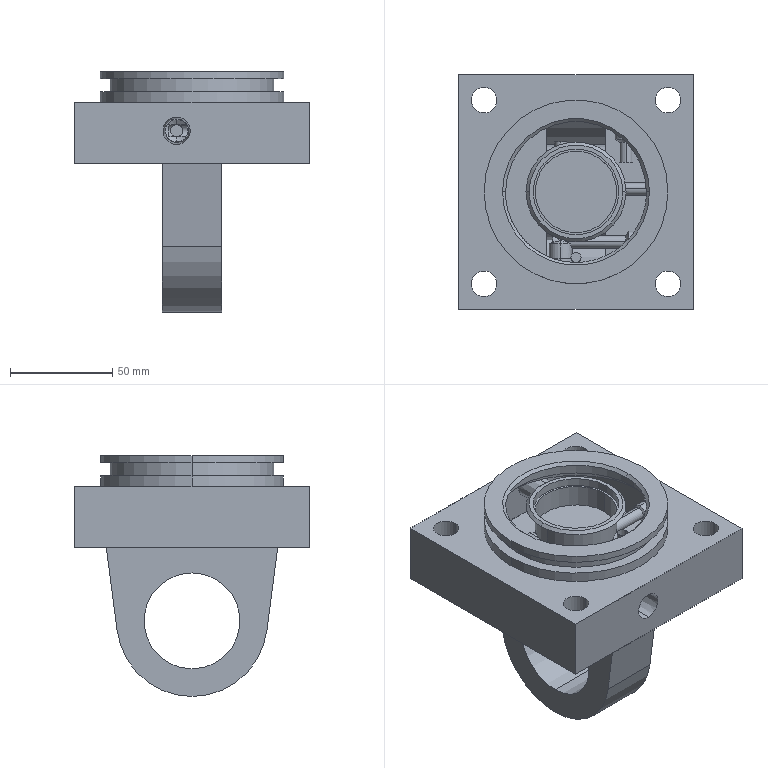Part | SolidWorks | features ICE 6, HoleWzd 4, Extrusion 1, RevCut 1 | 1 solid | 93 faces | box 115 x 115 x 118 mm | volume 524654 mm3 | cylinder 46 | plane 26 | cone 21 | commonest cylinder face diameters 6 x15 12.5 x8 10.7 x4 90 x4 5 x2 7.9 x2